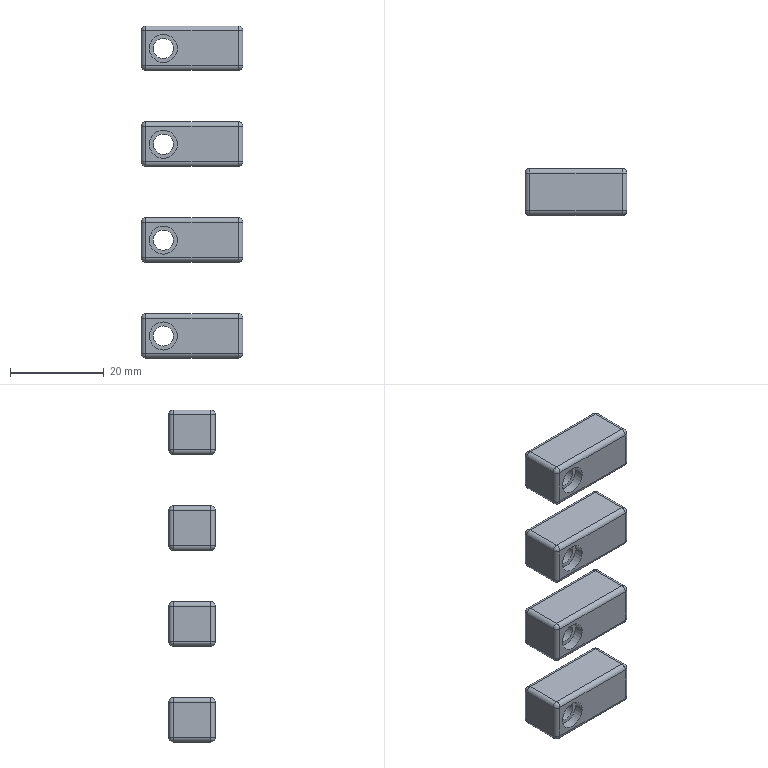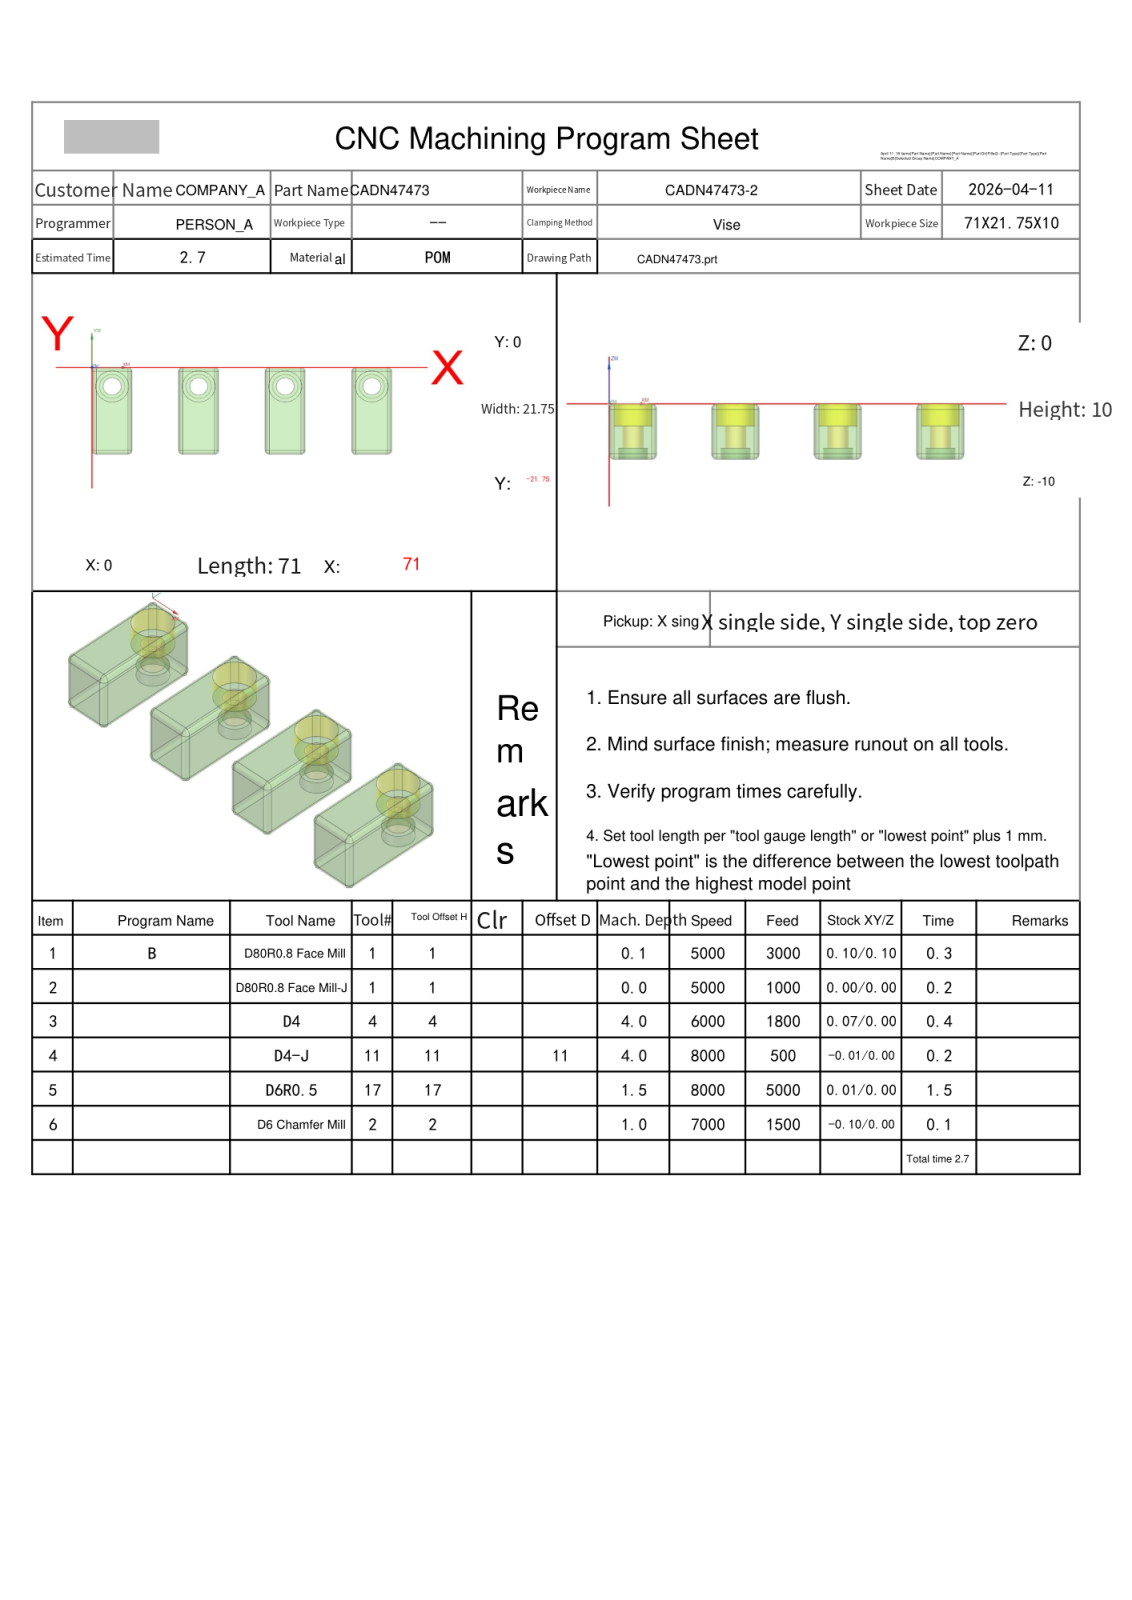NC program | NX | posted by the shop | part box 21.75 x 10 x 71 mm
Lines 260 to 1714 of 15118:
N5 T17 M06
(D6R0.5  D=6. R=0.5 H=17 ce=0.01 di=0.00)
G00 G90 G54 X11.16 Y-7.814 M03 S8000
G43 H17 Z20.
M08
Z1.5
G01 Y-20.913 Z.814 F5000.
X11.099 Y-21.337 Z.791
X10.971 Y-21.746 Z.769
X10.78 Y-22.129 Z.746
X10.529 Y-22.477 Z.724
X10.227 Y-22.779 Z.701
X9.879 Y-23.03 Z.679
X9.496 Y-23.221 Z.656
X9.087 Y-23.349 Z.634
X8.663 Y-23.41 Z.612
X.837 Z.201
X.413 Y-23.349 Z.179
X.004 Y-23.221 Z.156
X-.379 Y-23.03 Z.134
X-.727 Y-22.779 Z.112
X-1.029 Y-22.477 Z.089
X-1.28 Y-22.129 Z.067
X-1.471 Y-21.746 Z.044
X-1.599 Y-21.337 Z.022
X-1.66 Y-20.913 Z-.001
Y-20.75 Z-.009
Y-1.
G02 X1. Y1.66 I2.66 J0.0
G01 X8.5
G02 X11.16 Y-1. I0.0 J-2.66
G01 Y-20.75
G02 X8.5 Y-23.41 I-2.66 J0.0
G01 X1.
G02 X-1.66 Y-20.75 I0.0 J2.66
G01 X-1.676 Y-20.441
X-1.677 Y-20.133
X-1.678 Y-19.824
Y-19.516
X-1.679 Y-18.898 Z-.01
Y-18.281
X-1.683 Y-17.047
X-1.685 Y-15.813
X-1.689 Y-13.344 Z-.011
X-1.694 Y-10.875
X-1.698 Y-8.406 Z-.012
X-1.702 Y-5.938
X-1.707 Y-3.469 Z-.013
X-1.71 Y-1. Z-.014
Y-.918
X-1.706 Y-.836
X-1.7 Y-.755
X-1.691 Y-.673
X-1.681 Y-.592
X-1.667 Y-.511
X-1.651 Y-.431
X-1.633 Y-.351
X-1.612 Y-.272
X-1.589 Y-.193
X-1.564 Y-.115
X-1.536 Y-.038
X-1.506 Y.038
X-1.473 Y.113
X-1.439 Y.188
X-1.402 Y.261
X-1.363 Y.333
X-1.322 Y.403
X-1.279 Y.473
X-1.233 Y.541
X-1.186 Y.608
X-1.136 Y.673
X-1.085 Y.737
X-1.031 Y.8
X-.976 Y.86
X-.919 Y.919
X-.861 Y.977
X-.8 Y1.032
X-.738 Y1.085
X-.674 Y1.137
X-.609 Y1.187
X-.542 Y1.234
X-.474 Y1.28
X-.405 Y1.324
X-.334 Y1.365
X-.262 Y1.404
X-.189 Y1.442
X-.115 Y1.476
X-.039 Y1.509
X.037 Y1.539
X.114 Y1.568
X.192 Y1.593
X.271 Y1.617
X.35 Y1.638
X.43 Y1.656
X.51 Y1.672
X.591 Y1.686
X.672 Y1.697
X.754 Y1.706
X.836 Y1.712
X.918 Y1.716
X1. Y1.718
X2.587 Y1.72 Z-.015
X4.173 Y1.722
X4.796
X5.419 Y1.724
X6.96 Y1.727 Z-.016
X8.5 Y1.729
X8.582 Y1.728
X8.665 Y1.724
X8.747 Y1.718
X8.829 Y1.709
X8.911 Y1.699
X8.992 Y1.685
X9.073 Y1.669
X9.153 Y1.65
X9.233 Y1.63
X9.312 Y1.606
X9.391 Y1.581
X9.468 Y1.553
X9.545 Y1.523
X9.621 Y1.49
X9.695 Y1.455
X9.769 Y1.418
X9.842 Y1.379
X9.913 Y1.337
X9.983 Y1.294
X10.051 Y1.248
X10.119 Y1.2
X10.184 Y1.15 Z-.017
X10.249 Y1.099
X10.311 Y1.044
X10.373 Y.989
X10.432 Y.932
X10.489 Y.873
X10.545 Y.812
X10.599 Y.749
X10.651 Y.685
X10.701 Y.62
X10.749 Y.552
X10.795 Y.484
X10.838 Y.414
X10.881 Y.343
X10.92 Y.27
X10.958 Y.197
X10.992 Y.122
X11.026 Y.046
X11.056 Y-.031
X11.084 Y-.108
X11.11 Y-.187
X11.134 Y-.266
X11.154 Y-.346
X11.174 Y-.426
X11.189 Y-.507
X11.204 Y-.589
X11.214 Y-.67
X11.224 Y-.752
X11.229 Y-.835
X11.234 Y-.917
X11.235 Y-1.
X11.238 Y-3.469 Z-.018
X11.242 Y-5.938
X11.245 Y-8.406 Z-.019
X11.249 Y-10.875
X11.252 Y-13.344 Z-.02
X11.256 Y-15.813
X11.258 Y-18.281 Z-.021
X11.262 Y-20.75
X11.261 Y-20.833
X11.257 Y-20.917
X11.251 Y-21.
X11.242 Y-21.083
X11.231 Y-21.166
X11.217 Y-21.248
X11.201 Y-21.33
X11.182 Y-21.411
X11.162 Y-21.492 Z-.022
X11.138 Y-21.572
X11.112 Y-21.651
X11.084 Y-21.73
X11.053 Y-21.808
X11.02 Y-21.884
X10.985 Y-21.96
X10.947 Y-22.034
X10.907 Y-22.108
X10.865 Y-22.18
X10.821 Y-22.251
X10.775 Y-22.32
X10.726 Y-22.388
X10.676 Y-22.455
X10.624 Y-22.52
X10.569 Y-22.583
X10.513 Y-22.645
X10.455 Y-22.705
X10.395 Y-22.763
X10.333 Y-22.819
X10.27 Y-22.874
X10.205 Y-22.927
X10.139 Y-22.977
X10.071 Y-23.026
X10.002 Y-23.072
X9.931 Y-23.117
X9.859 Y-23.159
X9.785 Y-23.199
X9.711 Y-23.237
X9.635 Y-23.272
X9.559 Y-23.306
X9.481 Y-23.336
X9.402 Y-23.365
X9.323 Y-23.391
X9.243 Y-23.415
X9.162 Y-23.436
X9.081 Y-23.455
X8.999 Y-23.471
X8.916 Y-23.486
X8.833 Y-23.497
X8.75 Y-23.506
X8.667 Y-23.512
X8.584 Y-23.516
X8.5 Y-23.517
X6.625 Y-23.519 Z-.023
X4.75 Y-23.522
X2.875 Y-23.524 Z-.024
X1. Y-23.526
X.916
X.832 Y-23.521
X.749 Y-23.516
X.665 Y-23.506
X.582 Y-23.496
X.499 Y-23.481
X.417 Y-23.466
X.335 Y-23.446
X.254 Y-23.426
X.174 Y-23.401
X.094 Y-23.376
X.015 Y-23.347
X-.063 Y-23.317
X-.14 Y-23.283
X-.216 Y-23.248
X-.291 Y-23.21
X-.365 Y-23.17
X-.437 Y-23.127
X-.509 Y-23.083
X-.578 Y-23.036
X-.647 Y-22.988
X-.714 Y-22.937
X-.779 Y-22.885
X-.843 Y-22.83
X-.905 Y-22.774
X-.965 Y-22.715
X-1.024 Y-22.655
X-1.08 Y-22.593
X-1.135 Y-22.53
X-1.188 Y-22.464
X-1.239 Y-22.398 Z-.025
X-1.287 Y-22.329
X-1.335 Y-22.259
X-1.379 Y-22.188
X-1.422 Y-22.116
X-1.461 Y-22.042
X-1.5 Y-21.967
X-1.535 Y-21.891
X-1.569 Y-21.814
X-1.6 Y-21.736
X-1.629 Y-21.657
X-1.655 Y-21.577
X-1.679 Y-21.497
X-1.7 Y-21.415
X-1.719 Y-21.334
X-1.735 Y-21.251
X-1.75 Y-21.169
X-1.761 Y-21.085
X-1.77 Y-21.002
X-1.776 Y-20.918
X-1.781 Y-20.834
X-1.78 Y-20.75
X-1.785 Y-18.281 Z-.026
X-1.79 Y-15.813
X-1.794 Y-13.344 Z-.027
X-1.798 Y-10.875 Z-.028
X-1.802 Y-8.406 Z-.029
X-1.805 Y-5.938
X-1.809 Y-3.469 Z-.03
X-1.813 Y-1. Z-.031
X-1.809 Y-.842
X-1.796 Y-.685
X-1.774 Y-.529
X-1.743 Y-.374
X-1.704 Y-.221
X-1.656 Y-.071
X-1.6 Y.077
X-1.536 Y.221
X-1.464 Y.362
X-1.384 Y.498
X-1.296 Y.629 Z-.032
X-1.201 Y.755
X-1.1 Y.876
X-.991 Y.991
X-.877 Y1.1
X-.756 Y1.202
X-.63 Y1.297
X-.499 Y1.385
X-.363 Y1.466
X-.222 Y1.538
X-.078 Y1.603
X.069 Y1.66
X.22 Y1.708
X.373 Y1.748
X.528 Y1.779
X.684 Y1.801
X.842 Y1.815
X1. Y1.819
X2.875 Y1.822 Z-.033
X4.75 Y1.824 Z-.034
X6.625 Y1.828
X8.5 Y1.831 Z-.035
X8.659 Y1.826
X8.817 Y1.813
X8.974 Y1.791
X9.13 Y1.76
X9.284 Y1.721
X9.435 Y1.673
X9.584 Y1.616
X9.729 Y1.552
X9.87 Y1.479
X10.007 Y1.398
X10.139 Y1.31
X10.266 Y1.215
X10.388 Y1.113
X10.504 Y1.004
X10.613 Y.888
X10.716 Y.767
X10.811 Y.64
X10.9 Y.508 Z-.036
X10.981 Y.371
X11.054 Y.23
X11.119 Y.085
X11.176 Y-.064
X11.225 Y-.215
X11.264 Y-.369
X11.296 Y-.525
X11.318 Y-.682
X11.332 Y-.841
X11.336 Y-1.
X11.34 Y-3.469 Z-.037
X11.343 Y-5.938 Z-.038
X11.347 Y-8.406
X11.35 Y-10.875 Z-.039
X11.353 Y-13.344 Z-.04
X11.356 Y-15.813 Z-.041
X11.359 Y-18.281
X11.363 Y-20.75 Z-.042
X11.358 Y-20.911
X11.345 Y-21.071
X11.323 Y-21.23
X11.292 Y-21.387
X11.252 Y-21.543
X11.203 Y-21.696
X11.146 Y-21.846
X11.081 Y-21.993 Z-.043
X11.007 Y-22.136
X10.926 Y-22.274
X10.837 Y-22.408
X10.74 Y-22.537
X10.637 Y-22.659
X10.526 Y-22.776
X10.41 Y-22.887
X10.287 Y-22.991
X10.159 Y-23.088
X10.025 Y-23.177
X9.887 Y-23.259
X9.744 Y-23.333
X9.597 Y-23.399
X9.447 Y-23.456
X9.294 Y-23.505
X9.138 Y-23.546
X8.98 Y-23.577
X8.821 Y-23.6
X8.661 Y-23.614
X8.5 Y-23.619 Z-.044
X6.625 Y-23.621
X4.75 Y-23.623 Z-.045
X2.875 Y-23.625
X1. Y-23.627 Z-.046
X.839 Y-23.623
X.678 Y-23.61
X.518 Y-23.588
X.36 Y-23.556
X.203 Y-23.516
X.049 Y-23.467
X-.102 Y-23.41
X-.249 Y-23.344
X-.393 Y-23.27
X-.532 Y-23.188
X-.666 Y-23.099
X-.796 Y-23.002
X-.919 Y-22.898
X-1.037 Y-22.787 Z-.047
X-1.148 Y-22.669
X-1.252 Y-22.546
X-1.35 Y-22.417
X-1.439 Y-22.283
X-1.522 Y-22.144
X-1.596 Y-22.
X-1.662 Y-21.853
X-1.72 Y-21.702
X-1.77 Y-21.548
X-1.81 Y-21.391
X-1.842 Y-21.233
X-1.864 Y-21.073
X-1.873 Y-20.992
X-1.878 Y-20.912
X-1.882 Y-20.831
X-1.878 Y-20.75
X-1.887 Y-18.281 Z-.048
X-1.891 Y-15.813 Z-.049
X-1.894 Y-13.344 Z-.05
X-1.898 Y-10.875 Z-.051
X-1.902 Y-8.406 Z-.052
X-1.905 Y-5.938 Z-.053
X-1.909 Y-3.469 Z-.054
X-1.912 Y-1. Z-.055
X-1.908 Y-.837
X-1.894 Y-.674
X-1.872 Y-.512
X-1.84 Y-.352
X-1.799 Y-.193
X-1.75 Y-.038
X-1.692 Y.115
X-1.625 Y.264
X-1.551 Y.41 Z-.056
X-1.468 Y.55
X-1.377 Y.687
X-1.279 Y.817
X-1.174 Y.942
X-1.061 Y1.061
X-.943 Y1.174
X-.818 Y1.28
X-.687 Y1.378
X-.551 Y1.469
X-.411 Y1.553
X-.265 Y1.628
X-.116 Y1.695
X.037 Y1.753
X.192 Y1.803
X.351 Y1.844 Z-.057
X.511 Y1.877
X.673 Y1.9
X.836 Y1.914
X1. Y1.919
X2.875 Y1.921 Z-.058
X4.75 Y1.924
X6.625 Y1.927 Z-.059
X8.5 Y1.929 Z-.06
X8.664 Y1.924
X8.828 Y1.911
X8.991 Y1.888
X9.152 Y1.856
X9.311 Y1.815
X9.468 Y1.766
X9.621 Y1.707
X9.772 Y1.641
X9.918 Y1.565
X10.059 Y1.482
X10.196 Y1.391
X10.328 Y1.292 Z-.061
X10.454 Y1.186
X10.573 Y1.073
X10.686 Y.954
X10.793 Y.828
X10.892 Y.697
X10.983 Y.56
X11.067 Y.419
X11.143 Y.273
X11.21 Y.123
X11.269 Y-.031
X11.319 Y-.188
X11.361 Y-.347
X11.393 Y-.508
X11.416 Y-.671
X11.43 Y-.835
X11.435 Y-1. Z-.062
X11.438 Y-3.469 Z-.063
X11.441 Y-5.938
X11.445 Y-8.406 Z-.064
X11.448 Y-10.875 Z-.065
X11.451 Y-13.344 Z-.066
X11.454 Y-15.813 Z-.067
X11.457 Y-18.281 Z-.068
X11.46 Y-20.75 Z-.069
X11.456 Y-20.916
X11.442 Y-21.082
X11.419 Y-21.246 Z-.07
X11.387 Y-21.409
X11.346 Y-21.57
X11.296 Y-21.728
X11.236 Y-21.883
X11.169 Y-22.035
X11.093 Y-22.183
X11.008 Y-22.326
X10.916 Y-22.464
X10.817 Y-22.597
X10.709 Y-22.724
X10.595 Y-22.845
X10.475 Y-22.96
X10.348 Y-23.067
X10.215 Y-23.167
X10.077 Y-23.26
X9.934 Y-23.345 Z-.071
X9.786 Y-23.421
X9.635 Y-23.489
X9.479 Y-23.549
X9.321 Y-23.599
X9.16 Y-23.641
X8.997 Y-23.674
X8.832 Y-23.697
X8.666 Y-23.711
X8.5 Y-23.716
X6.625 Y-23.718 Z-.072
X4.75 Y-23.721 Z-.073
X2.875 Y-23.723
X1. Y-23.725 Z-.074
X.833 Y-23.721
X.667 Y-23.707
X.501 Y-23.684
X.338 Y-23.651
X.176 Y-23.61
X.017 Y-23.559
X-.139 Y-23.5 Z-.075
X-.292 Y-23.432
X-.44 Y-23.356
X-.584 Y-23.271
X-.723 Y-23.178
X-.857 Y-23.078
X-.984 Y-22.97
X-1.106 Y-22.856
X-1.221 Y-22.735
X-1.329 Y-22.607
X-1.429 Y-22.474
X-1.522 Y-22.335
X-1.607 Y-22.191
X-1.684 Y-22.043
X-1.753 Y-21.89
X-1.812 Y-21.734 Z-.076
X-1.863 Y-21.575
X-1.905 Y-21.413
X-1.938 Y-21.249
X-1.962 Y-21.084
X-1.976 Y-20.917
X-1.981 Y-20.75
X-1.985 Y-18.281 Z-.077
X-1.988 Y-15.813 Z-.078
X-1.992 Y-13.344 Z-.079
X-1.995 Y-10.875 Z-.081
X-1.998 Y-8.406 Z-.082
X-2.002 Y-5.938 Z-.083
X-2.005 Y-3.469 Z-.084
X-2.008 Y-1. Z-.085
X-2.004 Y-.831
X-1.99 Y-.663
X-1.967 Y-.496 Z-.086
X-1.934 Y-.33
X-1.892 Y-.167
X-1.841 Y-.006
X-1.781 Y.152
X-1.712 Y.306
X-1.635 Y.456
X-1.549 Y.602
X-1.456 Y.742
X-1.354 Y.877
X-1.245 Y1.007
X-1.129 Y1.129
X-1.007 Y1.246 Z-.087
X-.878 Y1.355
X-.743 Y1.457
X-.603 Y1.551
X-.457 Y1.637
X-.307 Y1.714
X-.153 Y1.784
X.005 Y1.844
X.166 Y1.896
X.329 Y1.938
X.495 Y1.972
X.663 Y1.995
X.831 Y2.01
X1. Y2.015 Z-.088
X2.875 Y2.017
X4.75 Y2.02 Z-.089
X6.625 Y2.022 Z-.09
X8.5 Y2.025 Z-.091
X8.67 Y2.02
X8.839 Y2.006
X9.007 Y1.983
X9.173 Y1.95
X9.338 Y1.908 Z-.092
X9.499 Y1.856
X9.658 Y1.796
X9.813 Y1.727
X9.964 Y1.649
X10.11 Y1.563
X10.252 Y1.469
X10.388 Y1.367
X10.517 Y1.257
X10.641 Y1.141
X10.758 Y1.018
X10.868 Y.888
X10.97 Y.752 Z-.093
X11.065 Y.611
X11.151 Y.465
X11.229 Y.314
X11.299 Y.159
X11.36 Y.001
X11.411 Y-.161
X11.454 Y-.326
X11.487 Y-.492
X11.511 Y-.661
X11.526 Y-.83
X11.531 Y-1.
X11.534 Y-3.469 Z-.095
X11.537 Y-5.938 Z-.096
X11.54 Y-8.406 Z-.097
X11.543 Y-10.875 Z-.098
X11.547 Y-13.344 Z-.099
X11.549 Y-15.813 Z-.1
X11.552 Y-18.281 Z-.102
X11.555 Y-20.75 Z-.103
Y-20.836
X11.551 Y-20.921
X11.545 Y-21.007
X11.537 Y-21.092
X11.513 Y-21.262
X11.48 Y-21.43
X11.437 Y-21.596
X11.385 Y-21.76
X11.324 Y-21.92
X11.254 Y-22.076
X11.176 Y-22.229 Z-.104
X11.089 Y-22.377
X10.994 Y-22.52
X10.891 Y-22.657
X10.78 Y-22.788
X10.663 Y-22.913
X10.538 Y-23.031
X10.407 Y-23.142
X10.27 Y-23.245
X10.128 Y-23.34
X9.98 Y-23.428
X9.828 Y-23.507
X9.671 Y-23.577 Z-.105
X9.511 Y-23.638
X9.347 Y-23.691
X9.181 Y-23.734
X9.013 Y-23.768
X8.843 Y-23.792
X8.672 Y-23.806
X8.5 Y-23.811
X6.625 Y-23.813 Z-.106
X4.75 Y-23.816 Z-.107
X2.875 Y-23.818 Z-.108
X1. Y-23.82 Z-.109
X.828 Y-23.816
X.656 Y-23.801
X.486 Y-23.778
X.317 Y-23.744
X.15 Y-23.701
X-.014 Y-23.649
X-.176 Y-23.588
X-.333 Y-23.518
X-.486 Y-23.439
X-.635 Y-23.351
X-.778 Y-23.256 Z-.11
X-.916 Y-23.152
X-1.048 Y-23.041
X-1.173 Y-22.923
X-1.292 Y-22.798
X-1.403 Y-22.666
X-1.507 Y-22.529
X-1.603 Y-22.385
X-1.691 Y-22.237
X-1.77 Y-22.084
X-1.841 Y-21.927
X-1.902 Y-21.766
X-1.955 Y-21.601 Z-.111
X-1.998 Y-21.434
X-2.032 Y-21.265
X-2.056 Y-21.094
X-2.071 Y-20.922
X-2.076 Y-20.75
X-2.079 Y-18.281 Z-.112
X-2.083 Y-15.813 Z-.114
X-2.086 Y-13.344 Z-.115
X-2.089 Y-10.875 Z-.116
X-2.093 Y-8.406 Z-.118
X-2.096 Y-5.938 Z-.119
X-2.099 Y-3.469 Z-.121
X-2.102 Y-1. Z-.122
X-2.101 Y-.913
X-2.098 Y-.826
X-2.092 Y-.739
X-2.083 Y-.653
X-2.072 Y-.566
X-2.059 Y-.48
X-2.043 Y-.395
X-2.025 Y-.31
X-2.005 Y-.225
X-1.982 Y-.141
X-1.957 Y-.058
X-1.929 Y.025 Z-.123
X-1.9 Y.107
X-1.867 Y.188
X-1.833 Y.268
X-1.796 Y.347
X-1.758 Y.425
X-1.717 Y.502
X-1.674 Y.577
X-1.628 Y.652
X-1.581 Y.725
X-1.532 Y.797
X-1.481 Y.867
X-1.427 Y.936
X-1.372 Y1.003
X-1.315 Y1.069
X-1.256 Y1.133
X-1.196 Y1.196
X-1.133 Y1.257
X-1.069 Y1.316
X-1.004 Y1.373
X-.936 Y1.428
X-.868 Y1.482 Z-.124
X-.797 Y1.533
X-.726 Y1.583
X-.653 Y1.63
X-.578 Y1.676
X-.503 Y1.719
X-.426 Y1.76
X-.348 Y1.799
X-.269 Y1.836
X-.189 Y1.87
X-.108 Y1.903
X-.026 Y1.933
X.056 Y1.961
X.14 Y1.986
X.224 Y2.009
X.309 Y2.03
X.394 Y2.048
X.479 Y2.064
X.566 Y2.077
X.652 Y2.088
X.826 Y2.103 Z-.125
X1. Y2.108
X2.875 Y2.111 Z-.126
X4.75 Y2.113 Z-.127
X6.625 Y2.116 Z-.128
X8.5 Y2.118 Z-.129
X8.675 Y2.113
X8.849 Y2.099
X9.022 Y2.075
X9.194 Y2.041
X9.363 Y1.997
X9.53 Y1.944
X9.694 Y1.882
X9.854 Y1.811 Z-.13
X10.009 Y1.731
X10.16 Y1.642
X10.306 Y1.545
X10.446 Y1.44
X10.58 Y1.327
X10.707 Y1.207
X10.827 Y1.08
X10.941 Y.946
X11.046 Y.806
X11.144 Y.661 Z-.131
X11.233 Y.51
X11.313 Y.355
X11.385 Y.195
X11.448 Y.031
X11.501 Y-.135
X11.545 Y-.305
X11.579 Y-.477
X11.604 Y-.65
X11.619 Y-.825
X11.624 Y-1. Z-.132
X11.627 Y-3.469 Z-.133
X11.63 Y-5.938 Z-.134
X11.633 Y-8.406 Z-.136
X11.636 Y-10.875 Z-.137
X11.639 Y-13.344 Z-.138
X11.642 Y-15.813 Z-.14
X11.645 Y-18.281 Z-.141
X11.648 Y-20.75 Z-.142
X11.647 Y-20.838 Z-.143
X11.643 Y-20.927
X11.637 Y-21.015
X11.628 Y-21.102
X11.618 Y-21.19
X11.604 Y-21.277
X11.588 Y-21.364
X11.57 Y-21.451
X11.549 Y-21.537
X11.526 Y-21.622
X11.5 Y-21.706
X11.472 Y-21.79
X11.41 Y-21.955
X11.338 Y-22.117
X11.257 Y-22.274
X11.167 Y-22.426
X11.069 Y-22.573 Z-.144
X10.963 Y-22.714
X10.849 Y-22.849
X10.728 Y-22.978
X10.6 Y-23.1
X10.465 Y-23.214
X10.324 Y-23.32
X10.177 Y-23.419
X10.025 Y-23.509
X9.868 Y-23.59
X9.706 Y-23.662 Z-.145
X9.541 Y-23.726
X9.373 Y-23.779
X9.202 Y-23.824
X9.028 Y-23.859
X8.853 Y-23.884
X8.677 Y-23.899
X8.5 Y-23.904
X6.625 Y-23.906 Z-.146
X4.75 Y-23.908 Z-.147
X2.875 Y-23.91 Z-.148
X1. Y-23.912 Z-.149
X.823 Y-23.908 Z-.15
X.646 Y-23.893
X.47 Y-23.868
X.296 Y-23.834
X.124 Y-23.79
X-.045 Y-23.736
X-.211 Y-23.673
X-.373 Y-23.601
X-.531 Y-23.519
X-.684 Y-23.429
X-.831 Y-23.331
X-.973 Y-23.224 Z-.151
X-1.109 Y-23.11
X-1.238 Y-22.988
X-1.36 Y-22.859
X-1.475 Y-22.724
X-1.582 Y-22.582
X-1.681 Y-22.434
X-1.771 Y-22.282
X-1.853 Y-22.124
X-1.89 Y-22.043
X-1.926 Y-21.962
X-1.959 Y-21.879 Z-.152
X-1.989 Y-21.796
X-2.017 Y-21.712
X-2.043 Y-21.627
X-2.067 Y-21.541
X-2.088 Y-21.455
X-2.107 Y-21.368
X-2.123 Y-21.281
X-2.137 Y-21.193
X-2.148 Y-21.105
X-2.163 Y-20.928
X-2.168 Y-20.75
X-2.171 Y-18.281 Z-.154
X-2.175 Y-15.813 Z-.155
X-2.178 Y-13.344 Z-.157
X-2.181 Y-10.875 Z-.158
X-2.184 Y-8.406 Z-.16
X-2.187 Y-5.938 Z-.162
X-2.19 Y-3.469 Z-.163
X-2.193 Y-1. Z-.165
X-2.192 Y-.91
X-2.188 Y-.821
X-2.182 Y-.732
X-2.173 Y-.642
X-2.162 Y-.554
X-2.148 Y-.465
X-2.133 Y-.377
X-2.114 Y-.289
X-2.093 Y-.202
X-2.069 Y-.116
X-2.044 Y-.03
X-2.015 Y.055
X-1.985 Y.139
X-1.951 Y.222
X-1.916 Y.305
X-1.878 Y.386 Z-.166
X-1.839 Y.466
X-1.796 Y.545
X-1.752 Y.623
X-1.705 Y.7
X-1.657 Y.775
X-1.606 Y.849
X-1.553 Y.922
X-1.498 Y.992
X-1.442 Y1.062
X-1.383 Y1.129
X-1.322 Y1.196
X-1.26 Y1.26
X-1.196 Y1.323
X-1.13 Y1.383
X-1.062 Y1.442
X-.993 Y1.499
X-.922 Y1.554
X-.85 Y1.607 Z-.167
X-.776 Y1.658
X-.701 Y1.707
X-.624 Y1.754
X-.547 Y1.798
X-.468 Y1.841
X-.387 Y1.881
X-.306 Y1.919
X-.224 Y1.954
X-.14 Y1.988
X-.056 Y2.018
X.029 Y2.047
X.115 Y2.073
X.201 Y2.097
X.288 Y2.118
X.376 Y2.137
X.464 Y2.153
X.553 Y2.167 Z-.168
X.642 Y2.179
X.731 Y2.188
X.821 Y2.194
X.91 Y2.198
X1. Y2.199
X2.875 Y2.202 Z-.169
X4.75 Y2.204 Z-.17
X6.625 Y2.206 Z-.171
X8.5 Y2.208 Z-.173
X8.59 Y2.207
X8.68 Y2.203
X8.77 Y2.197
X8.859 Y2.189
X8.949 Y2.177
X9.038 Y2.164
X9.126 Y2.147
X9.214 Y2.129
X9.302 Y2.108
X9.388 Y2.084
X9.475 Y2.058
X9.56 Y2.03
X9.645 Y1.999
X9.728 Y1.966
X9.811 Y1.93
X9.893 Y1.892
X9.973 Y1.852
X10.053 Y1.81 Z-.174
X10.131 Y1.765
X10.208 Y1.718
X10.284 Y1.67
X10.358 Y1.619
X10.431 Y1.566
X10.502 Y1.51
X10.572 Y1.453
X10.64 Y1.394
X10.706 Y1.334
X10.771 Y1.271
X10.834 Y1.206
X10.895 Y1.14
X10.954 Y1.072
X11.011 Y1.003
X11.066 Y.931
X11.12 Y.859
X11.171 Y.785 Z-.175
X11.22 Y.709
X11.267 Y.632
X11.312 Y.554
X11.354 Y.475
X11.395 Y.394
X11.433 Y.312
X11.468 Y.23
X11.502 Y.146
X11.533 Y.061
X11.561 Y-.024
X11.588 Y-.11
X11.612 Y-.197
X11.633 Y-.285
X11.652 Y-.373
X11.668 Y-.462
X11.682 Y-.551
X11.694 Y-.64
X11.703 Y-.73 Z-.176
X11.709 Y-.82
X11.713 Y-.91
X11.714 Y-1.
X11.717 Y-3.469 Z-.177
X11.72 Y-5.938 Z-.179
X11.723 Y-8.406 Z-.18
X11.726 Y-10.875 Z-.182
X11.729 Y-13.344 Z-.183
X11.731 Y-15.813 Z-.185
X11.734 Y-18.281 Z-.187
X11.737 Y-20.75 Z-.188
X11.736 Y-20.841
X11.732 Y-20.932
X11.726 Y-21.022
X11.717 Y-21.112
X11.706 Y-21.203
X11.692 Y-21.292 Z-.189
X11.676 Y-21.382
X11.657 Y-21.471
X11.636 Y-21.559
X11.612 Y-21.646
X11.586 Y-21.733
X11.557 Y-21.82
X11.526 Y-21.905
X11.492 Y-21.989
X11.456 Y-22.073
X11.418 Y-22.155
X11.378 Y-22.237
X11.335 Y-22.317
X11.29 Y-22.396
X11.243 Y-22.473
X11.194 Y-22.55
X11.142 Y-22.625
X11.089 Y-22.698
X11.033 Y-22.77 Z-.19
X10.975 Y-22.84
X10.916 Y-22.909
X10.854 Y-22.976
X10.791 Y-23.041
X10.726 Y-23.105
X10.659 Y-23.166
X10.591 Y-23.226
X10.52 Y-23.284
X10.449 Y-23.339
X10.375 Y-23.393
X10.301 Y-23.445
X10.224 Y-23.494
X10.147 Y-23.542
X10.068 Y-23.587
X9.988 Y-23.63
X9.906 Y-23.67
X9.824 Y-23.709 Z-.191
X9.74 Y-23.745
X9.656 Y-23.779
X9.571 Y-23.81
X9.485 Y-23.839
X9.397 Y-23.865
X9.31 Y-23.889
X9.221 Y-23.911
X9.133 Y-23.93
X9.043 Y-23.947
X8.953 Y-23.961
X8.863 Y-23.972
X8.773 Y-23.981
X8.682 Y-23.988
X8.591 Y-23.992
X8.5 Y-23.993
X6.625 Y-23.995 Z-.193
X4.75 Y-23.997 Z-.194
X2.875 Y-23.999 Z-.195
X1. Y-24.001 Z-.196
X.909 Y-24.
X.818 Y-23.997
X.727 Y-23.99
X.636 Y-23.981
X.545 Y-23.97
X.455 Y-23.956
X.366 Y-23.94 Z-.197
X.276 Y-23.921
X.188 Y-23.899
X.1 Y-23.875
X.012 Y-23.849
X-.074 Y-23.82
X-.16 Y-23.789
X-.245 Y-23.755
X-.329 Y-23.719
X-.411 Y-23.681
X-.493 Y-23.64
X-.574 Y-23.597
X-.653 Y-23.552
X-.731 Y-23.505
X-.808 Y-23.455
X-.883 Y-23.404
X-.957 Y-23.35
X-1.029 Y-23.294
X-1.099 Y-23.236 Z-.198
X-1.168 Y-23.176
X-1.236 Y-23.115
X-1.301 Y-23.051
X-1.365 Y-22.986
X-1.427 Y-22.919
X-1.487 Y-22.85
X-1.545 Y-22.779
X-1.601 Y-22.707
X-1.654 Y-22.633
X-1.706 Y-22.558
X-1.756 Y-22.482
X-1.804 Y-22.404
X-1.849 Y-22.325
X-1.892 Y-22.244
X-1.933 Y-22.162
X-1.972 Y-22.08
X-2.008 Y-21.996 Z-.199
X-2.042 Y-21.911
X-2.073 Y-21.825
X-2.102 Y-21.739
X-2.129 Y-21.651
X-2.153 Y-21.563
X-2.175 Y-21.475
X-2.194 Y-21.385
X-2.21 Y-21.295
X-2.225 Y-21.205
X-2.236 Y-21.115
X-2.245 Y-21.024
X-2.252 Y-20.933
X-2.256 Y-20.841
X-2.257 Y-20.75
X-2.26 Y-18.281 Z-.201
X-2.263 Y-15.813 Z-.203
X-2.266 Y-13.344 Z-.205
X-2.269 Y-10.875 Z-.206
X-2.272 Y-8.406 Z-.208
X-2.275 Y-5.938 Z-.21
X-2.278 Y-3.469 Z-.211
X-2.281 Y-1. Z-.213
X-2.276 Y-.828
X-2.263 Y-.657
X-2.241 Y-.487 Z-.214
X-2.21 Y-.318
X-2.17 Y-.151
X-2.121 Y.014
X-2.064 Y.176
X-1.998 Y.335
X-1.925 Y.49
X-1.843 Y.641
X-1.753 Y.788 Z-.215
X-1.656 Y.93
X-1.552 Y1.066
X-1.44 Y1.197
X-1.322 Y1.322
X-1.197 Y1.44
X-1.067 Y1.552
X-.93 Y1.657
X-.789 Y1.755 Z-.216
X-.642 Y1.845
X-.491 Y1.927
X-.336 Y2.001
X-.177 Y2.067
X-.015 Y2.125
X.15 Y2.174
X.317 Y2.214
X.486 Y2.246
X.656 Y2.268 Z-.217
X.828 Y2.282
X1. Y2.287
X2.875 Y2.289 Z-.218
X4.75 Y2.291 Z-.219
X6.625 Y2.293 Z-.221
X8.5 Y2.295 Z-.222
X8.672 Y2.291
X8.845 Y2.278
X9.016 Y2.255
X9.185 Y2.224 Z-.223
X9.353 Y2.184
X9.519 Y2.135
X9.681 Y2.078
X9.841 Y2.012
X9.997 Y1.938
X10.149 Y1.856
X10.296 Y1.766
X10.438 Y1.668 Z-.224
X10.575 Y1.563
X10.707 Y1.451
X10.832 Y1.332
X10.951 Y1.207
X11.064 Y1.076
X11.169 Y.939
X11.267 Y.797
X11.357 Y.65 Z-.225
X11.44 Y.498
X11.515 Y.342
X11.581 Y.183
X11.639 Y.02
X11.688 Y-.146
X11.728 Y-.314
X11.76 Y-.484
X11.783 Y-.655 Z-.226
X11.797 Y-.827
X11.801 Y-1.
X11.804 Y-3.469 Z-.228
X11.807 Y-5.938 Z-.229
X11.81 Y-8.406 Z-.231
X11.812 Y-10.875 Z-.233
X11.815 Y-13.344 Z-.234
X11.818 Y-15.813 Z-.236
X11.82 Y-18.281 Z-.238
X11.823 Y-20.75 Z-.24
X11.819 Y-20.924
X11.805 Y-21.097
X11.783 Y-21.27
X11.751 Y-21.441
X11.711 Y-21.61
X11.662 Y-21.777
X11.604 Y-21.941 Z-.241
X11.537 Y-22.102
X11.462 Y-22.259
X11.38 Y-22.413
X11.289 Y-22.561
X11.19 Y-22.705
X11.085 Y-22.843
X10.972 Y-22.975
X10.852 Y-23.102
X10.726 Y-23.222 Z-.242
X10.593 Y-23.335
X10.455 Y-23.441
X10.312 Y-23.54
X10.163 Y-23.631
X10.01 Y-23.715
X9.853 Y-23.79
X9.692 Y-23.857
X9.528 Y-23.915 Z-.243
X9.361 Y-23.965
X9.192 Y-24.005
X9.021 Y-24.037
X8.848 Y-24.06
X8.674 Y-24.074
X8.5 Y-24.079
X6.625 Y-24.081 Z-.245
X4.75 Y-24.083 Z-.246
X2.875 Y-24.085 Z-.247
X1. Y-24.087 Z-.249
X.825 Y-24.082
X.651 Y-24.069
X.478 Y-24.046
X.306 Y-24.015
X.136 Y-23.974
X-.032 Y-23.925
X-.196 Y-23.866
X-.358 Y-23.8 Z-.25
X-.516 Y-23.725
X-.669 Y-23.642
X-.819 Y-23.55
X-.963 Y-23.451
X-1.101 Y-23.345
X-1.235 Y-23.232
X-1.362 Y-23.111
X-1.482 Y-22.985 Z-.251
X-1.596 Y-22.852
X-1.702 Y-22.713
X-1.802 Y-22.569
X-1.893 Y-22.42
X-1.977 Y-22.267
X-2.052 Y-22.109
X-2.119 Y-21.947
X-2.178 Y-21.783 Z-.252
X-2.228 Y-21.615
X-2.269 Y-21.445
X-2.301 Y-21.273
X-2.324 Y-21.099
X-2.338 Y-20.925
X-2.343 Y-20.75
X-2.345 Y-18.281 Z-.254
X-2.348 Y-15.813 Z-.256
X-2.351 Y-13.344 Z-.258
X-2.354 Y-10.875 Z-.26
X-2.356 Y-8.406 Z-.262
X-2.359 Y-5.938 Z-.264
X-2.362 Y-3.469 Z-.266
X-2.365 Y-1. Z-.268
X-2.36 Y-.824
X-2.347 Y-.648
X-2.324 Y-.474
X-2.292 Y-.3
X-2.251 Y-.129
X-2.201 Y.04
X-2.143 Y.206
X-2.075 Y.369 Z-.269
X-2. Y.528
X-1.916 Y.683
X-1.824 Y.834
X-1.724 Y.979
X-1.617 Y1.119
X-1.503 Y1.253
X-1.381 Y1.381 Z-.27
X-1.254 Y1.503
X-1.12 Y1.618
X-.98 Y1.725
X-.835 Y1.825
X-.684 Y1.917
X-.529 Y2.002
X-.37 Y2.078 Z-.271
X-.207 Y2.146
X-.041 Y2.204
X.128 Y2.255
X.299 Y2.296
X.473 Y2.329
X.648 Y2.352
X.824 Y2.366
X1. Y2.371 Z-.272
X2.875 Y2.373 Z-.273
X4.75 Y2.375 Z-.274
X6.625 Y2.377 Z-.276
X8.5 Y2.379 Z-.277
X8.677 Y2.374 Z-.278
X8.853 Y2.361
X9.029 Y2.338
X9.203 Y2.306
X9.375 Y2.265
X9.545 Y2.215
X9.711 Y2.156
X9.875 Y2.088
X10.035 Y2.012 Z-.279
X10.19 Y1.928
X10.341 Y1.836
X10.487 Y1.736
X10.628 Y1.628
X10.763 Y1.513
X10.891 Y1.391
X11.013 Y1.263 Z-.28
X11.128 Y1.128
X11.236 Y.988
X11.337 Y.842
X11.43 Y.691
X11.514 Y.536
X11.591 Y.376
X11.659 Y.212 Z-.281
X11.718 Y.046
X11.768 Y-.124
X11.81 Y-.296
X11.842 Y-.471
X11.866 Y-.646
X11.88 Y-.823
X11.885 Y-1.
X11.887 Y-3.469 Z-.283
X11.89 Y-5.938 Z-.285
X11.892 Y-8.406 Z-.287
X11.895 Y-10.875 Z-.289
X11.897 Y-13.344 Z-.291
X11.9 Y-15.813 Z-.293
X11.903 Y-18.281 Z-.295
X11.906 Y-20.75 Z-.297
X11.901 Y-20.928
X11.887 Y-21.106
X11.864 Y-21.283
X11.832 Y-21.458
X11.79 Y-21.632
X11.74 Y-21.803 Z-.298
X11.68 Y-21.971
X11.612 Y-22.136
X11.536 Y-22.297
X11.451 Y-22.454
X11.358 Y-22.606
X11.257 Y-22.753
X11.148 Y-22.895 Z-.299
X11.033 Y-23.03
X10.91 Y-23.16
X10.781 Y-23.283
X10.645 Y-23.399
X10.504 Y-23.508
X10.357 Y-23.609
X10.205 Y-23.702
X10.048 Y-23.788 Z-.3
X9.887 Y-23.865
X9.722 Y-23.933
X9.554 Y-23.993
X9.383 Y-24.044
X9.209 Y-24.086
X9.033 Y-24.118
X8.857 Y-24.142 Z-.301
X8.678 Y-24.156
X8.5 Y-24.161
X6.625 Y-24.163 Z-.302
X4.75 Y-24.165 Z-.304
X2.875 Y-24.167 Z-.305
X1. Y-24.169 Z-.307
X.821 Y-24.164
X.643 Y-24.15
X.465 Y-24.127
X.289 Y-24.095
X.115 Y-24.053
X-.057 Y-24.002
X-.226 Y-23.943 Z-.308
X-.391 Y-23.874
X-.553 Y-23.797
X-.71 Y-23.712
X-.863 Y-23.619
X-1.011 Y-23.518
X-1.153 Y-23.409
X-1.289 Y-23.292 Z-.309
X-1.419 Y-23.169
X-1.543 Y-23.039
X-1.659 Y-22.903
X-1.768 Y-22.761
X-1.87 Y-22.614
X-1.964 Y-22.461
X-2.049 Y-22.304 Z-.31
X-2.127 Y-22.142
X-2.195 Y-21.977
X-2.255 Y-21.808
X-2.306 Y-21.636
X-2.349 Y-21.462
X-2.381 Y-21.286
X-2.405 Y-21.108
X-2.419 Y-20.929 Z-.311
X-2.424 Y-20.75
X-2.426 Y-18.281 Z-.313
X-2.429 Y-15.813 Z-.315
X-2.432 Y-13.344 Z-.317
X-2.435 Y-10.875 Z-.319
X-2.437 Y-8.406 Z-.321
X-2.44 Y-5.938 Z-.323
X-2.442 Y-3.469 Z-.325
X-2.445 Y-1. Z-.327
X-2.441 Y-.82
X-2.426 Y-.64 Z-.328
X-2.403 Y-.461
X-2.37 Y-.284
X-2.329 Y-.108
X-2.277 Y.065
X-2.217 Y.235
X-2.149 Y.402
X-2.071 Y.565 Z-.329
X-1.985 Y.723
X-1.891 Y.877
X-1.789 Y1.026
X-1.679 Y1.17
X-1.562 Y1.307
X-1.438 Y1.438 Z-.33
X-1.307 Y1.562
X-1.17 Y1.68
X-1.027 Y1.79
X-.878 Y1.892
X-.724 Y1.987
X-.566 Y2.073
X-.403 Y2.151 Z-.331
X-.236 Y2.22
X-.066 Y2.281
X.107 Y2.332
X.283 Y2.375
X.46 Y2.408
X.639 Y2.431
X.819 Y2.446 Z-.332
X1. Y2.451
X2.875 Y2.453 Z-.333
X4.75 Y2.455 Z-.335
X6.625 Y2.457 Z-.336
X8.5 Y2.458 Z-.338
X8.681 Y2.454
X8.862 Y2.44
X9.041 Y2.416 Z-.339
X9.219 Y2.384
X9.395 Y2.341
X9.569 Y2.29
X9.74 Y2.23
X9.907 Y2.161
X10.071 Y2.083
X10.23 Y1.997 Z-.34
X10.385 Y1.902
X10.534 Y1.8
X10.678 Y1.69
X10.816 Y1.572
X10.947 Y1.447
X11.072 Y1.316